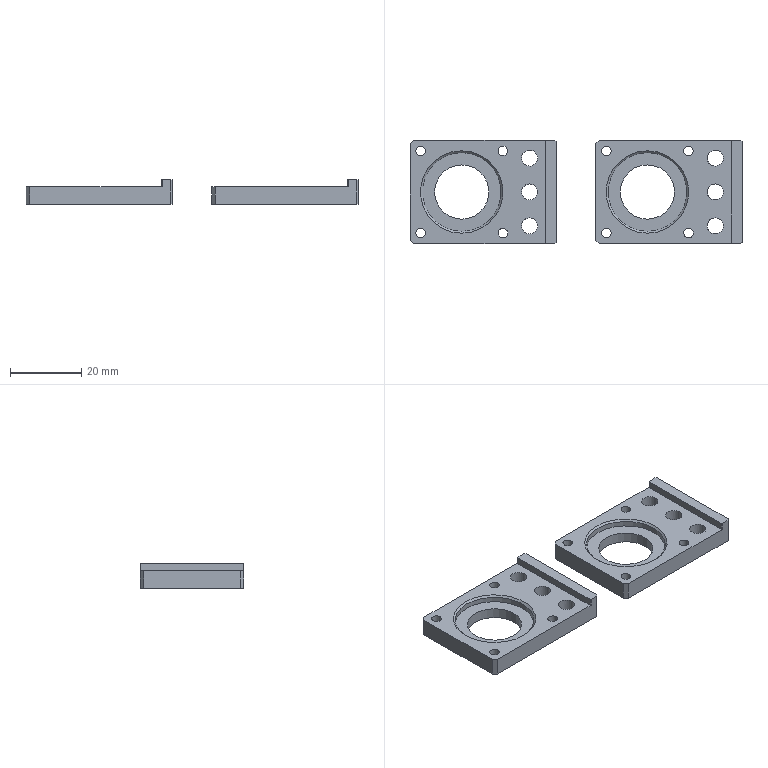CAM job | NX | 3-axis milling, drilling | part box 93 x 29 x 7 mm | stock box 98 x 30 x 10 mm
Tools:
number,name,description,diameter,corner_radius,flute_length,length,flutes
3,D3,平底铣刀-粗,3.0,0.0,20.0,75.0,2
8,D8,平底铣刀-粗,8.0,0.0,30.0,75.0,2
9,D10,平底铣刀-粗,10.0,0.0,35.0,75.0,2
7,D6-J,平底铣刀-精,6.0,0.0,25.0,75.0,2
10,D10-J,平底铣刀-精,10.0,0.0,35.0,75.0,2
1,D80R0.8飞刀,圆鼻刀-粗,80.0,0.8,50.0,75.0,2
1,D80R0.8飞刀-J,圆鼻刀-精,80.0,0.8,50.0,75.0,2
2,D6倒角刀,倒角刀,6.0,0.0,3.0,25.0,2
11,ZT4.5,钻头,4.5,0.0,35.0,50.0,2
17,ZT2.7,Drilling Tool,2.7,0.0,35.0,50.0,2
Operations:
program,operation,operation_type,tool,method,geometry_group,spindle_rpm,surface_speed,feed_per_tooth,feed_cut,feed_plunge,cut_length_mm,path_length_mm,cut_time_min,machine_time_min
B,底壁铣飞面一刀开粗_COPY,VolumeBased25DMillingOperation,D80R0.8飞刀,分层开粗-切深K-步距G,W-B,2800.0,703.696,0.5357,3000.0,100.0,1207.164,2296.186,0.4024,0.5113
B,底壁铣飞面一刀精光_COPY,VolumeBased25DMillingOperation,D80R0.8飞刀-J,侧刃精光-切深K-步距G,W-B,4000.0,1005.28,0.125,1000.0,100.0,200.998,236.998,0.201,0.2046
B,底壁铣分层开粗-中_COPY,VolumeBased25DMillingOperation,D10,分层开粗-切深K-步距G,W-B,8000.0,251.32,0.25,4000.0,100.0,2457.092,2650.925,0.6143,0.6337
B,孔粗_3,CylinderMilling,D10,METHOD,W-B,6000.0,157.0,0.25,3000.0,90.0,1088.09,1229.93,0.3632,0.3773
B,钻倒角_1,Operation,D6倒角刀,METHOD,W-B,8000.0,150.796,0.0625,1000.0,0.0,37.2,307.724,0.0372,0.0643
B,钻倒角_2,Operation,D6倒角刀,METHOD,W-B,8000.0,150.796,0.0625,1000.0,0.0,33.3,217.536,0.0333,0.0517
B,底壁铣倒角_COPY,VolumeBased25DMillingOperation,D6倒角刀,爬面_倒角-切深0-步距G,W-B,6500.0,122.519,0.1154,1500.0,100.0,144.718,280.768,0.0965,0.1101
B,平面去毛刺6X45L_COPY,SurfaceContour,D6倒角刀,爬面_倒角-切深0-步距G,W-B,6500.0,122.519,0.1154,1500.0,100.0,565.566,1323.277,0.377,0.4528
B,底壁铣精光底面-中_COPY,VolumeBased25DMillingOperation,D10-J,精光步距切深关,W-B,8000.0,251.32,0.0625,1000.0,100.0,263.082,289.682,0.2631,0.2657
B,底壁铣精光底面-中_COPY_1,VolumeBased25DMillingOperation,D10-J,精光步距切深关,W-B,8000.0,251.32,0.0625,1000.0,100.0,260.671,287.271,0.2607,0.2633
B,底壁铣精光侧面-中-选底面_COPY,VolumeBased25DMillingOperation,D10-J,侧刃精光-切深K-步距G,W-B,8000.0,251.32,0.0625,1000.0,100.0,48.323,75.923,0.0483,0.0511
B,底壁铣精光侧面-中-选底面_COPY_1,VolumeBased25DMillingOperation,D10-J,侧刃精光-切深K-步距G,W-B,8000.0,251.32,0.0625,1000.0,100.0,48.322,75.922,0.0483,0.0511
B,底壁铣精光侧面-中-选底面_COPY_2,VolumeBased25DMillingOperation,D10-J,侧刃精光-切深K-步距G,W-B,8000.0,251.32,0.0625,1000.0,100.0,96.545,217.221,0.0965,0.1086
A,顶面,FaceMilling,D80R0.8飞刀,侧刃精光-切深K-步距G,W-A,4000.0,1005.31,0.125,1000.0,100.0,187.0,223.0,0.187,0.1906
A,外形粗_2,VolumeBased25DMillingOperation,D10,METHOD,W-A,8000.0,251.327,0.3125,5000.0,80.0,3749.346,3893.246,0.7499,0.7643
A,沉头孔打点-深0.8,Operation,D6倒角刀,NONE,W-A,8000.0,150.796,0.0312,500.0,90.0,28.8,319.164,0.0576,0.0866
A,沉头孔-钻孔0段,Operation,ZT2.7,NONE,W-A,2800.0,23.75,0.0179,100.0,90.0,70.235,354.618,0.7024,0.7308
A,通孔-5-6,Operation,ZT4.5,NONE,W-A,3000.0,42.411,0.025,150.0,90.0,56.112,247.443,0.3741,0.3932
A,铣孔开粗D8_1,CylinderMilling,D8,NONE,W-A,8000.0,201.062,0.075,1200.0,100.0,963.249,1101.409,0.8027,0.8165
A,铣孔精光D8_1,CylinderMilling,D6-J,精光步距切深关,W-A,8000.0,201.062,0.0312,500.0,100.0,132.321,270.481,0.2646,0.2785
A,铣孔开粗D4_1,CylinderMilling,D3,NONE,W-A,8000.0,100.531,0.075,1200.0,100.0,1029.479,1532.479,0.8579,0.9082
A,铣孔精光D4_1,CylinderMilling,D3,精光步距切深关,W-A,8000.0,100.531,0.0312,500.0,100.0,88.483,591.483,0.177,0.2273
A,仅选体,SurfaceContour,D6倒角刀,METHOD,W-A,8000.0,150.796,0.1875,3000.0,100.0,408.666,636.173,0.1362,0.159
A,铣倒角_1,PlanarMilling,D6倒角刀,NONE,W-A,8000.0,150.796,0.0312,500.0,100.0,183.778,638.578,0.3676,0.413
A,铣倒角_2,PlanarMilling,D6倒角刀,METHOD,W-A,8000.0,150.796,0.0312,500.0,100.0,104.118,440.13,0.2082,0.2418
A,铣倒角_3,PlanarMilling,D6倒角刀,METHOD,W-A,8000.0,150.796,0.0625,1000.0,100.0,101.274,237.619,0.1013,0.1149
A,外形半精_2,VolumeBased25DMillingOperation,D10-J,METHOD,W-A,8000.0,251.327,0.0625,1000.0,100.0,358.2,411.6,0.3582,0.3635